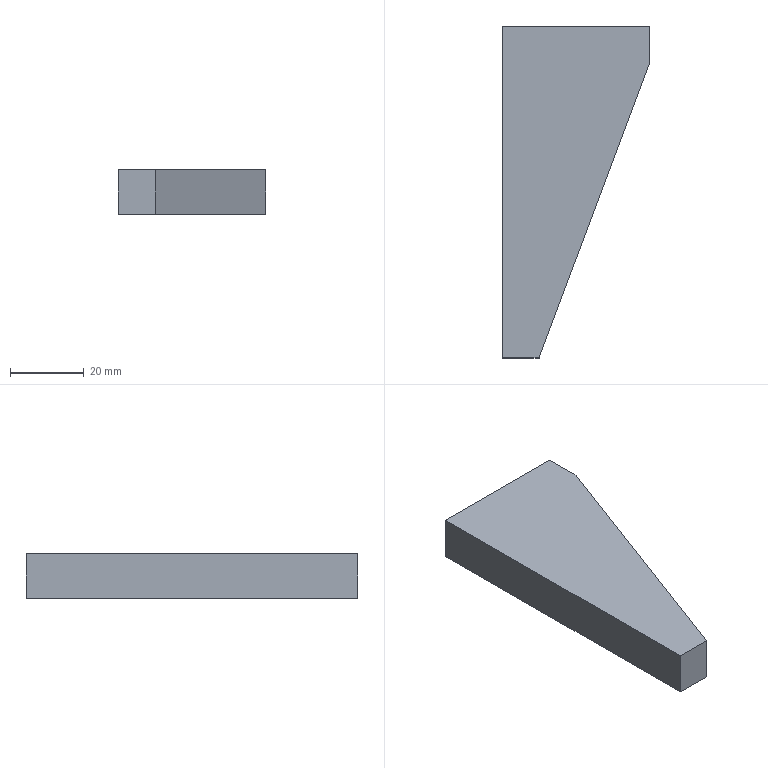Part | SolidWorks | features MBimport 1 | 1 solid | 7 faces | box 40 x 90 x 12 mm | volume 28800 mm3 | plane 7
STEP:
#1=CARTESIAN_POINT('',(63.623,86.988,0.));
#2=VERTEX_POINT('',#1);
#3=CARTESIAN_POINT('',(23.623,86.988,0.));
#4=VERTEX_POINT('',#3);
#5=CARTESIAN_POINT('',(63.623,86.988,0.));
#6=DIRECTION('',(-1.,0.,0.));
#7=VECTOR('',#6,1000.);
#8=LINE('',#5,#7);
#9=EDGE_CURVE('',#2,#4,#8,.T.);
#10=ORIENTED_EDGE('',*,*,#9,.F.);
#11=CARTESIAN_POINT('',(63.623,76.988,0.));
#12=VERTEX_POINT('',#11);
#13=CARTESIAN_POINT('',(63.623,76.988,0.));
#14=DIRECTION('',(0.,1.,0.));
#15=VECTOR('',#14,1000.);
#16=LINE('',#13,#15);
#17=EDGE_CURVE('',#12,#2,#16,.T.);
#18=ORIENTED_EDGE('',*,*,#17,.F.);
#19=CARTESIAN_POINT('',(33.623,-3.012,0.));
#20=VERTEX_POINT('',#19);
#21=CARTESIAN_POINT('',(33.623,-3.012,0.));
#22=DIRECTION('',(0.3511,0.9363,0.));
#23=VECTOR('',#22,1000.);
#24=LINE('',#21,#23);
#25=EDGE_CURVE('',#20,#12,#24,.T.);
#26=ORIENTED_EDGE('',*,*,#25,.F.);
#27=CARTESIAN_POINT('',(23.623,-3.012,0.));
#28=VERTEX_POINT('',#27);
#29=CARTESIAN_POINT('',(23.623,-3.012,0.));
#30=DIRECTION('',(1.,0.,0.));
#31=VECTOR('',#30,1000.);
#32=LINE('',#29,#31);
#33=EDGE_CURVE('',#28,#20,#32,.T.);
#34=ORIENTED_EDGE('',*,*,#33,.F.);
#35=CARTESIAN_POINT('',(23.623,86.988,0.));
#36=DIRECTION('',(0.,-1.,0.));
#37=VECTOR('',#36,1000.);
#38=LINE('',#35,#37);
#39=EDGE_CURVE('',#4,#28,#38,.T.);
#40=ORIENTED_EDGE('',*,*,#39,.F.);
#41=EDGE_LOOP('',(#10,#18,#26,#34,#40));
#42=FACE_OUTER_BOUND('',#41,.T.);
#43=CARTESIAN_POINT('',(0.,0.,0.));
#44=DIRECTION('',(0.,0.,1.));
#45=DIRECTION('',(1.,0.,0.));
#46=AXIS2_PLACEMENT_3D('',#43,#44,#45);
#47=PLANE('',#46);
#48=ADVANCED_FACE('',(#42),#47,.F.);
#49=CARTESIAN_POINT('',(63.623,86.988,12.));
#50=VERTEX_POINT('',#49);
#51=CARTESIAN_POINT('',(23.623,86.988,12.));
#52=VERTEX_POINT('',#51);
#53=CARTESIAN_POINT('',(63.623,86.988,12.));
#54=DIRECTION('',(-1.,0.,0.));
#55=VECTOR('',#54,1000.);
#56=LINE('',#53,#55);
#57=EDGE_CURVE('',#50,#52,#56,.T.);
#58=ORIENTED_EDGE('',*,*,#57,.T.);
#59=CARTESIAN_POINT('',(23.623,-3.012,12.));
#60=VERTEX_POINT('',#59);
#61=CARTESIAN_POINT('',(23.623,86.988,12.));
#62=DIRECTION('',(0.,-1.,0.));
#63=VECTOR('',#62,1000.);
#64=LINE('',#61,#63);
#65=EDGE_CURVE('',#52,#60,#64,.T.);
#66=ORIENTED_EDGE('',*,*,#65,.T.);
#67=CARTESIAN_POINT('',(33.623,-3.012,12.));
#68=VERTEX_POINT('',#67);
#69=CARTESIAN_POINT('',(23.623,-3.012,12.));
#70=DIRECTION('',(1.,0.,0.));
#71=VECTOR('',#70,1000.);
#72=LINE('',#69,#71);
#73=EDGE_CURVE('',#60,#68,#72,.T.);
#74=ORIENTED_EDGE('',*,*,#73,.T.);
#75=CARTESIAN_POINT('',(63.623,76.988,12.));
#76=VERTEX_POINT('',#75);
#77=CARTESIAN_POINT('',(33.623,-3.012,12.));
#78=DIRECTION('',(0.3511,0.9363,0.));
#79=VECTOR('',#78,1000.);
#80=LINE('',#77,#79);
#81=EDGE_CURVE('',#68,#76,#80,.T.);
#82=ORIENTED_EDGE('',*,*,#81,.T.);
#83=CARTESIAN_POINT('',(63.623,76.988,12.));
#84=DIRECTION('',(0.,1.,0.));
#85=VECTOR('',#84,1000.);
#86=LINE('',#83,#85);
#87=EDGE_CURVE('',#76,#50,#86,.T.);
#88=ORIENTED_EDGE('',*,*,#87,.T.);
#89=EDGE_LOOP('',(#58,#66,#74,#82,#88));
#90=FACE_OUTER_BOUND('',#89,.T.);
#91=CARTESIAN_POINT('',(0.,0.,12.));
#92=DIRECTION('',(0.,0.,1.));
#93=DIRECTION('',(1.,0.,0.));
#94=AXIS2_PLACEMENT_3D('',#91,#92,#93);
#95=PLANE('',#94);
#96=ADVANCED_FACE('',(#90),#95,.T.);
#97=ORIENTED_EDGE('',*,*,#17,.T.);
#98=CARTESIAN_POINT('',(63.623,86.988,12.));
#99=DIRECTION('',(0.,0.,-1.));
#100=VECTOR('',#99,1000.);
#101=LINE('',#98,#100);
#102=EDGE_CURVE('',#50,#2,#101,.T.);
#103=ORIENTED_EDGE('',*,*,#102,.F.);
#104=ORIENTED_EDGE('',*,*,#87,.F.);
#105=CARTESIAN_POINT('',(63.623,76.988,12.));
#106=DIRECTION('',(0.,0.,-1.));
#107=VECTOR('',#106,1000.);
#108=LINE('',#105,#107);
#109=EDGE_CURVE('',#76,#12,#108,.T.);
#110=ORIENTED_EDGE('',*,*,#109,.T.);
#111=EDGE_LOOP('',(#97,#103,#104,#110));
#112=FACE_OUTER_BOUND('',#111,.T.);
#113=CARTESIAN_POINT('',(63.623,76.988,12.));
#114=DIRECTION('',(-1.,0.,0.));
#115=DIRECTION('',(0.,0.,1.));
#116=AXIS2_PLACEMENT_3D('',#113,#114,#115);
#117=PLANE('',#116);
#118=ADVANCED_FACE('',(#112),#117,.F.);
#119=ORIENTED_EDGE('',*,*,#25,.T.);
#120=ORIENTED_EDGE('',*,*,#109,.F.);
#121=ORIENTED_EDGE('',*,*,#81,.F.);
#122=CARTESIAN_POINT('',(33.623,-3.012,12.));
#123=DIRECTION('',(0.,0.,-1.));
#124=VECTOR('',#123,1000.);
#125=LINE('',#122,#124);
#126=EDGE_CURVE('',#68,#20,#125,.T.);
#127=ORIENTED_EDGE('',*,*,#126,.T.);
#128=EDGE_LOOP('',(#119,#120,#121,#127));
#129=FACE_OUTER_BOUND('',#128,.T.);
#130=CARTESIAN_POINT('',(33.623,-3.012,12.));
#131=DIRECTION('',(-0.9363,0.3511,0.));
#132=DIRECTION('',(0.,0.,1.));
#133=AXIS2_PLACEMENT_3D('',#130,#131,#132);
#134=PLANE('',#133);
#135=ADVANCED_FACE('',(#129),#134,.F.);
#136=ORIENTED_EDGE('',*,*,#33,.T.);
#137=ORIENTED_EDGE('',*,*,#126,.F.);
#138=ORIENTED_EDGE('',*,*,#73,.F.);
#139=CARTESIAN_POINT('',(23.623,-3.012,12.));
#140=DIRECTION('',(0.,0.,-1.));
#141=VECTOR('',#140,1000.);
#142=LINE('',#139,#141);
#143=EDGE_CURVE('',#60,#28,#142,.T.);
#144=ORIENTED_EDGE('',*,*,#143,.T.);
#145=EDGE_LOOP('',(#136,#137,#138,#144));
#146=FACE_OUTER_BOUND('',#145,.T.);
#147=CARTESIAN_POINT('',(23.623,-3.012,12.));
#148=DIRECTION('',(0.,1.,0.));
#149=DIRECTION('',(1.,0.,0.));
#150=AXIS2_PLACEMENT_3D('',#147,#148,#149);
#151=PLANE('',#150);
#152=ADVANCED_FACE('',(#146),#151,.F.);
#153=ORIENTED_EDGE('',*,*,#39,.T.);
#154=ORIENTED_EDGE('',*,*,#143,.F.);
#155=ORIENTED_EDGE('',*,*,#65,.F.);
#156=CARTESIAN_POINT('',(23.623,86.988,12.));
#157=DIRECTION('',(0.,0.,-1.));
#158=VECTOR('',#157,1000.);
#159=LINE('',#156,#158);
#160=EDGE_CURVE('',#52,#4,#159,.T.);
#161=ORIENTED_EDGE('',*,*,#160,.T.);
#162=EDGE_LOOP('',(#153,#154,#155,#161));
#163=FACE_OUTER_BOUND('',#162,.T.);
#164=CARTESIAN_POINT('',(23.623,86.988,12.));
#165=DIRECTION('',(1.,0.,0.));
#166=DIRECTION('',(0.,1.,0.));
#167=AXIS2_PLACEMENT_3D('',#164,#165,#166);
#168=PLANE('',#167);
#169=ADVANCED_FACE('',(#163),#168,.F.);
#170=ORIENTED_EDGE('',*,*,#9,.T.);
#171=ORIENTED_EDGE('',*,*,#160,.F.);
#172=ORIENTED_EDGE('',*,*,#57,.F.);
#173=ORIENTED_EDGE('',*,*,#102,.T.);
#174=EDGE_LOOP('',(#170,#171,#172,#173));
#175=FACE_OUTER_BOUND('',#174,.T.);
#176=CARTESIAN_POINT('',(63.623,86.988,12.));
#177=DIRECTION('',(0.,-1.,0.));
#178=DIRECTION('',(0.,0.,-1.));
#179=AXIS2_PLACEMENT_3D('',#176,#177,#178);
#180=PLANE('',#179);
#181=ADVANCED_FACE('',(#175),#180,.F.);
#182=CLOSED_SHELL('',(#48,#96,#118,#135,#152,#169,#181));
#183=MANIFOLD_SOLID_BREP('',#182);
#184=CARTESIAN_POINT('',(0.,0.,0.));
#185=DIRECTION('',(0.,0.,1.));
#186=DIRECTION('',(1.,0.,0.));
#187=AXIS2_PLACEMENT_3D('',#184,#185,#186);
#188=(LENGTH_UNIT()NAMED_UNIT(*)SI_UNIT(.MILLI.,.METRE.));
#189=UNCERTAINTY_MEASURE_WITH_UNIT(LENGTH_MEASURE(0.00001),#188,'','');
#190=(NAMED_UNIT(*)PLANE_ANGLE_UNIT()SI_UNIT($,.RADIAN.));
#191=(NAMED_UNIT(*)SI_UNIT($,.STERADIAN.)SOLID_ANGLE_UNIT());
#192=(GEOMETRIC_REPRESENTATION_CONTEXT(3)GLOBAL_UNCERTAINTY_ASSIGNED_CONTEXT((#189))GLOBAL_UNIT_ASSIGNED_CONTEXT((#188,#190,#191))REPRESENTATION_CONTEXT('',''));
#193=ADVANCED_BREP_SHAPE_REPRESENTATION('',(#183,#187),#192);